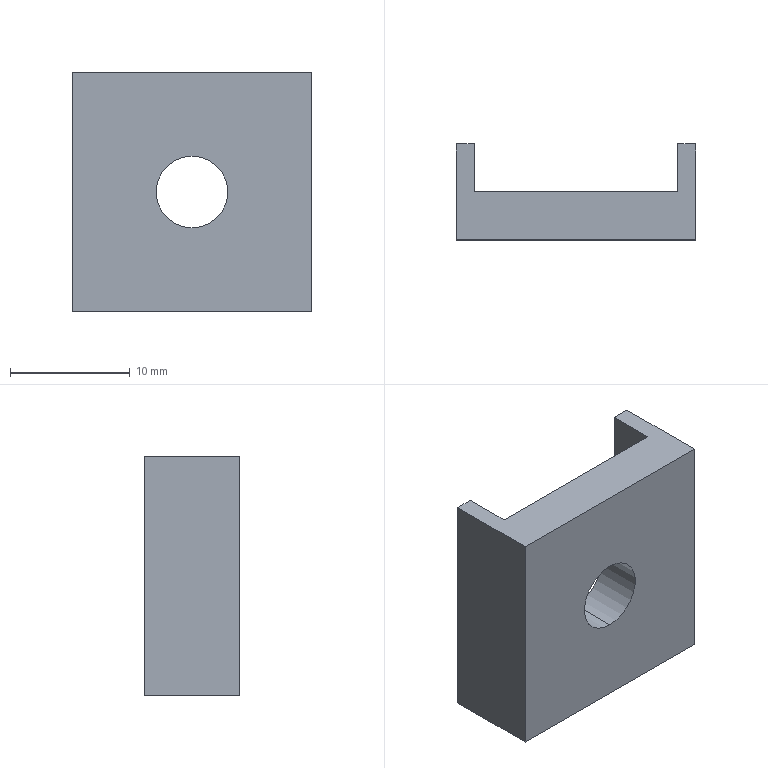Part | STEP file | 开关-2 | 1 solid | 12 faces | box 20 x 8 x 20 mm | volume 1727 mm3 | plane 10 | cylinder 2 | commonest cylinder face diameters 6 x2
STEP:
#1=CARTESIAN_POINT('',(0.,0.,0.));
#2=DIRECTION('',(0.,0.,1.));
#3=DIRECTION('',(1.,0.,0.));
#4=AXIS2_PLACEMENT_3D('',#1,#2,#3);
#5=CARTESIAN_POINT('',(0.,4.,-3.));
#6=VERTEX_POINT('',#5);
#7=CARTESIAN_POINT('',(0.,0.,-3.));
#8=VERTEX_POINT('',#7);
#9=CARTESIAN_POINT('',(0.,8.001,-3.));
#10=DIRECTION('',(0.,-1.,0.));
#11=VECTOR('',#10,1.);
#12=LINE('',#9,#11);
#13=CARTESIAN_POINT('',(0.,8.001,0.));
#14=DIRECTION('',(0.,-1.,0.));
#15=DIRECTION('',(0.,0.,-1.));
#16=AXIS2_PLACEMENT_3D('',#13,#14,#15);
#17=CYLINDRICAL_SURFACE('',#16,3.);
#18=CARTESIAN_POINT('',(6.283,0.));
#19=DIRECTION('',(0.,1.));
#20=VECTOR('',#19,1.);
#21=LINE('',#18,#20);
#22=(GEOMETRIC_REPRESENTATION_CONTEXT(2)PARAMETRIC_REPRESENTATION_CONTEXT()REPRESENTATION_CONTEXT('',''));
#23=DEFINITIONAL_REPRESENTATION('',(#21),#22);
#24=PCURVE('',#17,#23);
#25=CARTESIAN_POINT('',(0.,8.001,0.));
#26=DIRECTION('',(0.,-1.,0.));
#27=DIRECTION('',(0.,0.,-1.));
#28=AXIS2_PLACEMENT_3D('',#25,#26,#27);
#29=CYLINDRICAL_SURFACE('',#28,3.);
#30=CARTESIAN_POINT('',(0.,0.));
#31=DIRECTION('',(0.,1.));
#32=VECTOR('',#31,1.);
#33=LINE('',#30,#32);
#34=(GEOMETRIC_REPRESENTATION_CONTEXT(2)PARAMETRIC_REPRESENTATION_CONTEXT()REPRESENTATION_CONTEXT('',''));
#35=DEFINITIONAL_REPRESENTATION('',(#33),#34);
#36=PCURVE('',#29,#35);
#37=SURFACE_CURVE('',#12,(#24,#36),.PCURVE_S1.);
#38=EDGE_CURVE('',#6,#8,#37,.T.);
#39=ORIENTED_EDGE('',*,*,#38,.T.);
#40=CARTESIAN_POINT('',(0.,0.,3.));
#41=VERTEX_POINT('',#40);
#42=CARTESIAN_POINT('',(0.,0.,0.));
#43=DIRECTION('',(0.,-1.,0.));
#44=DIRECTION('',(0.,0.,-1.));
#45=AXIS2_PLACEMENT_3D('',#42,#43,#44);
#46=CIRCLE('',#45,3.);
#47=CARTESIAN_POINT('',(0.,8.001));
#48=DIRECTION('',(1.,0.));
#49=VECTOR('',#48,1.);
#50=LINE('',#47,#49);
#51=(GEOMETRIC_REPRESENTATION_CONTEXT(2)PARAMETRIC_REPRESENTATION_CONTEXT()REPRESENTATION_CONTEXT('',''));
#52=DEFINITIONAL_REPRESENTATION('',(#50),#51);
#53=PCURVE('',#17,#52);
#54=CARTESIAN_POINT('',(0.,0.,0.));
#55=DIRECTION('',(0.,-1.,0.));
#56=DIRECTION('',(0.,0.,-1.));
#57=AXIS2_PLACEMENT_3D('',#54,#55,#56);
#58=PLANE('',#57);
#59=CARTESIAN_POINT('',(0.,0.));
#60=DIRECTION('',(1.,0.));
#61=AXIS2_PLACEMENT_2D('',#59,#60);
#62=CIRCLE('',#61,3.);
#63=(GEOMETRIC_REPRESENTATION_CONTEXT(2)PARAMETRIC_REPRESENTATION_CONTEXT()REPRESENTATION_CONTEXT('',''));
#64=DEFINITIONAL_REPRESENTATION('',(#62),#63);
#65=PCURVE('',#58,#64);
#66=SURFACE_CURVE('',#46,(#53,#65),.PCURVE_S1.);
#67=EDGE_CURVE('',#41,#8,#66,.T.);
#68=ORIENTED_EDGE('',*,*,#67,.F.);
#69=CARTESIAN_POINT('',(0.,4.,3.));
#70=VERTEX_POINT('',#69);
#71=CARTESIAN_POINT('',(0.,8.001,3.));
#72=DIRECTION('',(0.,-1.,0.));
#73=VECTOR('',#72,1.);
#74=LINE('',#71,#73);
#75=CARTESIAN_POINT('',(3.142,0.));
#76=DIRECTION('',(0.,1.));
#77=VECTOR('',#76,1.);
#78=LINE('',#75,#77);
#79=(GEOMETRIC_REPRESENTATION_CONTEXT(2)PARAMETRIC_REPRESENTATION_CONTEXT()REPRESENTATION_CONTEXT('',''));
#80=DEFINITIONAL_REPRESENTATION('',(#78),#79);
#81=PCURVE('',#17,#80);
#82=CARTESIAN_POINT('',(3.142,0.));
#83=DIRECTION('',(0.,1.));
#84=VECTOR('',#83,1.);
#85=LINE('',#82,#84);
#86=(GEOMETRIC_REPRESENTATION_CONTEXT(2)PARAMETRIC_REPRESENTATION_CONTEXT()REPRESENTATION_CONTEXT('',''));
#87=DEFINITIONAL_REPRESENTATION('',(#85),#86);
#88=PCURVE('',#29,#87);
#89=SURFACE_CURVE('',#74,(#81,#88),.PCURVE_S1.);
#90=EDGE_CURVE('',#70,#41,#89,.T.);
#91=ORIENTED_EDGE('',*,*,#90,.F.);
#92=CARTESIAN_POINT('',(0.,4.,0.));
#93=DIRECTION('',(0.,1.,0.));
#94=DIRECTION('',(0.,0.,-1.));
#95=AXIS2_PLACEMENT_3D('',#92,#93,#94);
#96=CIRCLE('',#95,3.);
#97=CARTESIAN_POINT('',(6.283,4.001));
#98=DIRECTION('',(-1.,0.));
#99=VECTOR('',#98,1.);
#100=LINE('',#97,#99);
#101=(GEOMETRIC_REPRESENTATION_CONTEXT(2)PARAMETRIC_REPRESENTATION_CONTEXT()REPRESENTATION_CONTEXT('',''));
#102=DEFINITIONAL_REPRESENTATION('',(#100),#101);
#103=PCURVE('',#17,#102);
#104=CARTESIAN_POINT('',(-8.5,4.,-10.));
#105=DIRECTION('',(0.,-1.,0.));
#106=DIRECTION('',(0.,0.,-1.));
#107=AXIS2_PLACEMENT_3D('',#104,#105,#106);
#108=PLANE('',#107);
#109=CARTESIAN_POINT('',(-7.,8.5));
#110=CARTESIAN_POINT('',(-7.,3.304));
#111=CARTESIAN_POINT('',(-11.5,5.902));
#112=CARTESIAN_POINT('',(-16.,8.5));
#113=CARTESIAN_POINT('',(-11.5,11.098));
#114=CARTESIAN_POINT('',(-7.,13.696));
#115=CARTESIAN_POINT('',(-7.,8.5));
#116=(BOUNDED_CURVE()B_SPLINE_CURVE(2,(#109,#110,#111,#112,#113,#114,#115),.UNSPECIFIED.,.T.,.F.)B_SPLINE_CURVE_WITH_KNOTS((1,2,2,2,2,1),(-2.094,0.,2.094,4.189,6.283,8.378),.UNSPECIFIED.)CURVE()GEOMETRIC_REPRESENTATION_ITEM()RATIONAL_B_SPLINE_CURVE((1.,0.5,1.,0.5,1.,0.5,1.))REPRESENTATION_ITEM(''));
#117=(GEOMETRIC_REPRESENTATION_CONTEXT(2)PARAMETRIC_REPRESENTATION_CONTEXT()REPRESENTATION_CONTEXT('',''));
#118=DEFINITIONAL_REPRESENTATION('',(#116),#117);
#119=PCURVE('',#108,#118);
#120=SURFACE_CURVE('',#96,(#103,#119),.PCURVE_S1.);
#121=EDGE_CURVE('',#6,#70,#120,.T.);
#122=ORIENTED_EDGE('',*,*,#121,.F.);
#123=EDGE_LOOP('',(#39,#68,#91,#122));
#124=FACE_BOUND('',#123,.F.);
#125=ADVANCED_FACE('',(#124),#17,.F.);
#126=CARTESIAN_POINT('',(-10.,8.,10.));
#127=VERTEX_POINT('',#126);
#128=CARTESIAN_POINT('',(-8.5,8.,10.));
#129=VERTEX_POINT('',#128);
#130=CARTESIAN_POINT('',(-10.,8.,10.));
#131=DIRECTION('',(1.,0.,0.));
#132=VECTOR('',#131,1.);
#133=LINE('',#130,#132);
#134=CARTESIAN_POINT('',(0.,8.,0.));
#135=DIRECTION('',(0.,-1.,0.));
#136=DIRECTION('',(0.,0.,-1.));
#137=AXIS2_PLACEMENT_3D('',#134,#135,#136);
#138=PLANE('',#137);
#139=CARTESIAN_POINT('',(-10.,-10.));
#140=DIRECTION('',(0.,1.));
#141=VECTOR('',#140,1.);
#142=LINE('',#139,#141);
#143=(GEOMETRIC_REPRESENTATION_CONTEXT(2)PARAMETRIC_REPRESENTATION_CONTEXT()REPRESENTATION_CONTEXT('',''));
#144=DEFINITIONAL_REPRESENTATION('',(#142),#143);
#145=PCURVE('',#138,#144);
#146=CARTESIAN_POINT('',(-10.,8.,10.));
#147=DIRECTION('',(0.,0.,-1.));
#148=DIRECTION('',(-1.,0.,0.));
#149=AXIS2_PLACEMENT_3D('',#146,#147,#148);
#150=PLANE('',#149);
#151=CARTESIAN_POINT('',(0.,0.));
#152=DIRECTION('',(-1.,0.));
#153=VECTOR('',#152,1.);
#154=LINE('',#151,#153);
#155=(GEOMETRIC_REPRESENTATION_CONTEXT(2)PARAMETRIC_REPRESENTATION_CONTEXT()REPRESENTATION_CONTEXT('',''));
#156=DEFINITIONAL_REPRESENTATION('',(#154),#155);
#157=PCURVE('',#150,#156);
#158=SURFACE_CURVE('',#133,(#145,#157),.PCURVE_S1.);
#159=EDGE_CURVE('',#127,#129,#158,.T.);
#160=ORIENTED_EDGE('',*,*,#159,.T.);
#161=CARTESIAN_POINT('',(-8.5,8.,-10.));
#162=VERTEX_POINT('',#161);
#163=CARTESIAN_POINT('',(-8.5,8.,-10.));
#164=DIRECTION('',(0.,0.,1.));
#165=VECTOR('',#164,1.);
#166=LINE('',#163,#165);
#167=CARTESIAN_POINT('',(10.,-8.5));
#168=DIRECTION('',(-1.,0.));
#169=VECTOR('',#168,1.);
#170=LINE('',#167,#169);
#171=(GEOMETRIC_REPRESENTATION_CONTEXT(2)PARAMETRIC_REPRESENTATION_CONTEXT()REPRESENTATION_CONTEXT('',''));
#172=DEFINITIONAL_REPRESENTATION('',(#170),#171);
#173=PCURVE('',#138,#172);
#174=CARTESIAN_POINT('',(-8.5,8.,-10.));
#175=DIRECTION('',(-1.,0.,0.));
#176=DIRECTION('',(0.,0.,1.));
#177=AXIS2_PLACEMENT_3D('',#174,#175,#176);
#178=PLANE('',#177);
#179=CARTESIAN_POINT('',(0.,0.));
#180=DIRECTION('',(1.,0.));
#181=VECTOR('',#180,1.);
#182=LINE('',#179,#181);
#183=(GEOMETRIC_REPRESENTATION_CONTEXT(2)PARAMETRIC_REPRESENTATION_CONTEXT()REPRESENTATION_CONTEXT('',''));
#184=DEFINITIONAL_REPRESENTATION('',(#182),#183);
#185=PCURVE('',#178,#184);
#186=SURFACE_CURVE('',#166,(#173,#185),.PCURVE_S1.);
#187=EDGE_CURVE('',#162,#129,#186,.T.);
#188=ORIENTED_EDGE('',*,*,#187,.F.);
#189=CARTESIAN_POINT('',(-10.,8.,-10.));
#190=VERTEX_POINT('',#189);
#191=CARTESIAN_POINT('',(-10.,8.,-10.));
#192=DIRECTION('',(-1.,0.,0.));
#193=VECTOR('',#192,1.);
#194=LINE('',#191,#193);
#195=CARTESIAN_POINT('',(10.,-10.));
#196=DIRECTION('',(0.,-1.));
#197=VECTOR('',#196,1.);
#198=LINE('',#195,#197);
#199=(GEOMETRIC_REPRESENTATION_CONTEXT(2)PARAMETRIC_REPRESENTATION_CONTEXT()REPRESENTATION_CONTEXT('',''));
#200=DEFINITIONAL_REPRESENTATION('',(#198),#199);
#201=PCURVE('',#138,#200);
#202=CARTESIAN_POINT('',(-10.,8.,-10.));
#203=DIRECTION('',(0.,0.,1.));
#204=DIRECTION('',(1.,0.,0.));
#205=AXIS2_PLACEMENT_3D('',#202,#203,#204);
#206=PLANE('',#205);
#207=CARTESIAN_POINT('',(0.,0.));
#208=DIRECTION('',(-1.,0.));
#209=VECTOR('',#208,1.);
#210=LINE('',#207,#209);
#211=(GEOMETRIC_REPRESENTATION_CONTEXT(2)PARAMETRIC_REPRESENTATION_CONTEXT()REPRESENTATION_CONTEXT('',''));
#212=DEFINITIONAL_REPRESENTATION('',(#210),#211);
#213=PCURVE('',#206,#212);
#214=SURFACE_CURVE('',#194,(#201,#213),.PCURVE_S1.);
#215=EDGE_CURVE('',#162,#190,#214,.T.);
#216=ORIENTED_EDGE('',*,*,#215,.T.);
#217=CARTESIAN_POINT('',(-10.,8.,10.));
#218=DIRECTION('',(0.,0.,1.));
#219=VECTOR('',#218,1.);
#220=LINE('',#217,#219);
#221=CARTESIAN_POINT('',(-10.,-10.));
#222=DIRECTION('',(-1.,0.));
#223=VECTOR('',#222,1.);
#224=LINE('',#221,#223);
#225=(GEOMETRIC_REPRESENTATION_CONTEXT(2)PARAMETRIC_REPRESENTATION_CONTEXT()REPRESENTATION_CONTEXT('',''));
#226=DEFINITIONAL_REPRESENTATION('',(#224),#225);
#227=PCURVE('',#138,#226);
#228=CARTESIAN_POINT('',(-10.,8.,10.));
#229=DIRECTION('',(1.,0.,0.));
#230=DIRECTION('',(0.,0.,-1.));
#231=AXIS2_PLACEMENT_3D('',#228,#229,#230);
#232=PLANE('',#231);
#233=CARTESIAN_POINT('',(0.,0.));
#234=DIRECTION('',(-1.,0.));
#235=VECTOR('',#234,1.);
#236=LINE('',#233,#235);
#237=(GEOMETRIC_REPRESENTATION_CONTEXT(2)PARAMETRIC_REPRESENTATION_CONTEXT()REPRESENTATION_CONTEXT('',''));
#238=DEFINITIONAL_REPRESENTATION('',(#236),#237);
#239=PCURVE('',#232,#238);
#240=SURFACE_CURVE('',#220,(#227,#239),.PCURVE_S1.);
#241=EDGE_CURVE('',#190,#127,#240,.T.);
#242=ORIENTED_EDGE('',*,*,#241,.T.);
#243=EDGE_LOOP('',(#160,#188,#216,#242));
#244=FACE_BOUND('',#243,.T.);
#245=ADVANCED_FACE('',(#244),#138,.F.);
#246=CARTESIAN_POINT('',(10.,0.,10.));
#247=VERTEX_POINT('',#246);
#248=CARTESIAN_POINT('',(10.,0.,-10.));
#249=VERTEX_POINT('',#248);
#250=CARTESIAN_POINT('',(10.,0.,10.));
#251=DIRECTION('',(0.,0.,-1.));
#252=VECTOR('',#251,1.);
#253=LINE('',#250,#252);
#254=CARTESIAN_POINT('',(10.,8.,10.));
#255=DIRECTION('',(-1.,0.,0.));
#256=DIRECTION('',(0.,0.,1.));
#257=AXIS2_PLACEMENT_3D('',#254,#255,#256);
#258=PLANE('',#257);
#259=CARTESIAN_POINT('',(0.,-8.));
#260=DIRECTION('',(-1.,0.));
#261=VECTOR('',#260,1.);
#262=LINE('',#259,#261);
#263=(GEOMETRIC_REPRESENTATION_CONTEXT(2)PARAMETRIC_REPRESENTATION_CONTEXT()REPRESENTATION_CONTEXT('',''));
#264=DEFINITIONAL_REPRESENTATION('',(#262),#263);
#265=PCURVE('',#258,#264);
#266=CARTESIAN_POINT('',(-10.,10.));
#267=DIRECTION('',(1.,0.));
#268=VECTOR('',#267,1.);
#269=LINE('',#266,#268);
#270=(GEOMETRIC_REPRESENTATION_CONTEXT(2)PARAMETRIC_REPRESENTATION_CONTEXT()REPRESENTATION_CONTEXT('',''));
#271=DEFINITIONAL_REPRESENTATION('',(#269),#270);
#272=PCURVE('',#58,#271);
#273=SURFACE_CURVE('',#253,(#265,#272),.PCURVE_S1.);
#274=EDGE_CURVE('',#247,#249,#273,.T.);
#275=ORIENTED_EDGE('',*,*,#274,.T.);
#276=CARTESIAN_POINT('',(10.,8.,-10.));
#277=VERTEX_POINT('',#276);
#278=CARTESIAN_POINT('',(10.,8.,-10.));
#279=DIRECTION('',(0.,-1.,0.));
#280=VECTOR('',#279,1.);
#281=LINE('',#278,#280);
#282=CARTESIAN_POINT('',(-20.,0.));
#283=DIRECTION('',(0.,-1.));
#284=VECTOR('',#283,1.);
#285=LINE('',#282,#284);
#286=(GEOMETRIC_REPRESENTATION_CONTEXT(2)PARAMETRIC_REPRESENTATION_CONTEXT()REPRESENTATION_CONTEXT('',''));
#287=DEFINITIONAL_REPRESENTATION('',(#285),#286);
#288=PCURVE('',#258,#287);
#289=CARTESIAN_POINT('',(20.,0.));
#290=DIRECTION('',(0.,-1.));
#291=VECTOR('',#290,1.);
#292=LINE('',#289,#291);
#293=(GEOMETRIC_REPRESENTATION_CONTEXT(2)PARAMETRIC_REPRESENTATION_CONTEXT()REPRESENTATION_CONTEXT('',''));
#294=DEFINITIONAL_REPRESENTATION('',(#292),#293);
#295=PCURVE('',#206,#294);
#296=SURFACE_CURVE('',#281,(#288,#295),.PCURVE_S1.);
#297=EDGE_CURVE('',#277,#249,#296,.T.);
#298=ORIENTED_EDGE('',*,*,#297,.F.);
#299=CARTESIAN_POINT('',(10.,8.,10.));
#300=VERTEX_POINT('',#299);
#301=CARTESIAN_POINT('',(10.,8.,10.));
#302=DIRECTION('',(0.,0.,-1.));
#303=VECTOR('',#302,1.);
#304=LINE('',#301,#303);
#305=CARTESIAN_POINT('',(0.,0.));
#306=DIRECTION('',(-1.,0.));
#307=VECTOR('',#306,1.);
#308=LINE('',#305,#307);
#309=(GEOMETRIC_REPRESENTATION_CONTEXT(2)PARAMETRIC_REPRESENTATION_CONTEXT()REPRESENTATION_CONTEXT('',''));
#310=DEFINITIONAL_REPRESENTATION('',(#308),#309);
#311=PCURVE('',#258,#310);
#312=CARTESIAN_POINT('',(0.,8.,0.));
#313=DIRECTION('',(0.,-1.,0.));
#314=DIRECTION('',(0.,0.,-1.));
#315=AXIS2_PLACEMENT_3D('',#312,#313,#314);
#316=PLANE('',#315);
#317=CARTESIAN_POINT('',(-10.,10.));
#318=DIRECTION('',(1.,0.));
#319=VECTOR('',#318,1.);
#320=LINE('',#317,#319);
#321=(GEOMETRIC_REPRESENTATION_CONTEXT(2)PARAMETRIC_REPRESENTATION_CONTEXT()REPRESENTATION_CONTEXT('',''));
#322=DEFINITIONAL_REPRESENTATION('',(#320),#321);
#323=PCURVE('',#316,#322);
#324=SURFACE_CURVE('',#304,(#311,#323),.PCURVE_S1.);
#325=EDGE_CURVE('',#300,#277,#324,.T.);
#326=ORIENTED_EDGE('',*,*,#325,.F.);
#327=CARTESIAN_POINT('',(10.,8.,10.));
#328=DIRECTION('',(0.,-1.,0.));
#329=VECTOR('',#328,1.);
#330=LINE('',#327,#329);
#331=CARTESIAN_POINT('',(0.,0.));
#332=DIRECTION('',(0.,-1.));
#333=VECTOR('',#332,1.);
#334=LINE('',#331,#333);
#335=(GEOMETRIC_REPRESENTATION_CONTEXT(2)PARAMETRIC_REPRESENTATION_CONTEXT()REPRESENTATION_CONTEXT('',''));
#336=DEFINITIONAL_REPRESENTATION('',(#334),#335);
#337=PCURVE('',#258,#336);
#338=CARTESIAN_POINT('',(-20.,0.));
#339=DIRECTION('',(0.,-1.));
#340=VECTOR('',#339,1.);
#341=LINE('',#338,#340);
#342=(GEOMETRIC_REPRESENTATION_CONTEXT(2)PARAMETRIC_REPRESENTATION_CONTEXT()REPRESENTATION_CONTEXT('',''));
#343=DEFINITIONAL_REPRESENTATION('',(#341),#342);
#344=PCURVE('',#150,#343);
#345=SURFACE_CURVE('',#330,(#337,#344),.PCURVE_S1.);
#346=EDGE_CURVE('',#300,#247,#345,.T.);
#347=ORIENTED_EDGE('',*,*,#346,.T.);
#348=EDGE_LOOP('',(#275,#298,#326,#347));
#349=FACE_BOUND('',#348,.T.);
#350=ADVANCED_FACE('',(#349),#258,.F.);
#351=ORIENTED_EDGE('',*,*,#215,.F.);
#352=CARTESIAN_POINT('',(-8.5,4.,-10.));
#353=VERTEX_POINT('',#352);
#354=CARTESIAN_POINT('',(-8.5,8.,-10.));
#355=DIRECTION('',(0.,-1.,0.));
#356=VECTOR('',#355,1.);
#357=LINE('',#354,#356);
#358=CARTESIAN_POINT('',(1.5,0.));
#359=DIRECTION('',(0.,-1.));
#360=VECTOR('',#359,1.);
#361=LINE('',#358,#360);
#362=(GEOMETRIC_REPRESENTATION_CONTEXT(2)PARAMETRIC_REPRESENTATION_CONTEXT()REPRESENTATION_CONTEXT('',''));
#363=DEFINITIONAL_REPRESENTATION('',(#361),#362);
#364=PCURVE('',#206,#363);
#365=CARTESIAN_POINT('',(0.,0.));
#366=DIRECTION('',(0.,-1.));
#367=VECTOR('',#366,1.);
#368=LINE('',#365,#367);
#369=(GEOMETRIC_REPRESENTATION_CONTEXT(2)PARAMETRIC_REPRESENTATION_CONTEXT()REPRESENTATION_CONTEXT('',''));
#370=DEFINITIONAL_REPRESENTATION('',(#368),#369);
#371=PCURVE('',#178,#370);
#372=SURFACE_CURVE('',#357,(#364,#371),.PCURVE_S1.);
#373=EDGE_CURVE('',#162,#353,#372,.T.);
#374=ORIENTED_EDGE('',*,*,#373,.T.);
#375=CARTESIAN_POINT('',(8.5,4.,-10.));
#376=VERTEX_POINT('',#375);
#377=CARTESIAN_POINT('',(-8.5,4.,-10.));
#378=DIRECTION('',(1.,0.,0.));
#379=VECTOR('',#378,1.);
#380=LINE('',#377,#379);
#381=CARTESIAN_POINT('',(1.5,-4.));
#382=DIRECTION('',(1.,0.));
#383=VECTOR('',#382,1.);
#384=LINE('',#381,#383);
#385=(GEOMETRIC_REPRESENTATION_CONTEXT(2)PARAMETRIC_REPRESENTATION_CONTEXT()REPRESENTATION_CONTEXT('',''));
#386=DEFINITIONAL_REPRESENTATION('',(#384),#385);
#387=PCURVE('',#206,#386);
#388=CARTESIAN_POINT('',(0.,0.));
#389=DIRECTION('',(0.,1.));
#390=VECTOR('',#389,1.);
#391=LINE('',#388,#390);
#392=(GEOMETRIC_REPRESENTATION_CONTEXT(2)PARAMETRIC_REPRESENTATION_CONTEXT()REPRESENTATION_CONTEXT('',''));
#393=DEFINITIONAL_REPRESENTATION('',(#391),#392);
#394=PCURVE('',#108,#393);
#395=SURFACE_CURVE('',#380,(#387,#394),.PCURVE_S1.);
#396=EDGE_CURVE('',#353,#376,#395,.T.);
#397=ORIENTED_EDGE('',*,*,#396,.T.);
#398=CARTESIAN_POINT('',(8.5,8.,-10.));
#399=VERTEX_POINT('',#398);
#400=CARTESIAN_POINT('',(8.5,8.,-10.));
#401=DIRECTION('',(0.,1.,0.));
#402=VECTOR('',#401,1.);
#403=LINE('',#400,#402);
#404=CARTESIAN_POINT('',(18.5,0.));
#405=DIRECTION('',(0.,1.));
#406=VECTOR('',#405,1.);
#407=LINE('',#404,#406);
#408=(GEOMETRIC_REPRESENTATION_CONTEXT(2)PARAMETRIC_REPRESENTATION_CONTEXT()REPRESENTATION_CONTEXT('',''));
#409=DEFINITIONAL_REPRESENTATION('',(#407),#408);
#410=PCURVE('',#206,#409);
#411=CARTESIAN_POINT('',(8.5,8.,-10.));
#412=DIRECTION('',(1.,0.,0.));
#413=DIRECTION('',(0.,0.,-1.));
#414=AXIS2_PLACEMENT_3D('',#411,#412,#413);
#415=PLANE('',#414);
#416=CARTESIAN_POINT('',(0.,0.));
#417=DIRECTION('',(0.,1.));
#418=VECTOR('',#417,1.);
#419=LINE('',#416,#418);
#420=(GEOMETRIC_REPRESENTATION_CONTEXT(2)PARAMETRIC_REPRESENTATION_CONTEXT()REPRESENTATION_CONTEXT('',''));
#421=DEFINITIONAL_REPRESENTATION('',(#419),#420);
#422=PCURVE('',#415,#421);
#423=SURFACE_CURVE('',#403,(#410,#422),.PCURVE_S1.);
#424=EDGE_CURVE('',#376,#399,#423,.T.);
#425=ORIENTED_EDGE('',*,*,#424,.T.);
#426=CARTESIAN_POINT('',(-10.,8.,-10.));
#427=DIRECTION('',(-1.,0.,0.));
#428=VECTOR('',#427,1.);
#429=LINE('',#426,#428);
#430=CARTESIAN_POINT('',(0.,0.));
#431=DIRECTION('',(-1.,0.));
#432=VECTOR('',#431,1.);
#433=LINE('',#430,#432);
#434=(GEOMETRIC_REPRESENTATION_CONTEXT(2)PARAMETRIC_REPRESENTATION_CONTEXT()REPRESENTATION_CONTEXT('',''));
#435=DEFINITIONAL_REPRESENTATION('',(#433),#434);
#436=PCURVE('',#206,#435);
#437=CARTESIAN_POINT('',(10.,-10.));
#438=DIRECTION('',(0.,-1.));
#439=VECTOR('',#438,1.);
#440=LINE('',#437,#439);
#441=(GEOMETRIC_REPRESENTATION_CONTEXT(2)PARAMETRIC_REPRESENTATION_CONTEXT()REPRESENTATION_CONTEXT('',''));
#442=DEFINITIONAL_REPRESENTATION('',(#440),#441);
#443=PCURVE('',#316,#442);
#444=SURFACE_CURVE('',#429,(#436,#443),.PCURVE_S1.);
#445=EDGE_CURVE('',#277,#399,#444,.T.);
#446=ORIENTED_EDGE('',*,*,#445,.F.);
#447=ORIENTED_EDGE('',*,*,#297,.T.);
#448=CARTESIAN_POINT('',(-10.,0.,-10.));
#449=VERTEX_POINT('',#448);
#450=CARTESIAN_POINT('',(-10.,0.,-10.));
#451=DIRECTION('',(-1.,0.,0.));
#452=VECTOR('',#451,1.);
#453=LINE('',#450,#452);
#454=CARTESIAN_POINT('',(0.,-8.));
#455=DIRECTION('',(-1.,0.));
#456=VECTOR('',#455,1.);
#457=LINE('',#454,#456);
#458=(GEOMETRIC_REPRESENTATION_CONTEXT(2)PARAMETRIC_REPRESENTATION_CONTEXT()REPRESENTATION_CONTEXT('',''));
#459=DEFINITIONAL_REPRESENTATION('',(#457),#458);
#460=PCURVE('',#206,#459);
#461=CARTESIAN_POINT('',(10.,-10.));
#462=DIRECTION('',(0.,-1.));
#463=VECTOR('',#462,1.);
#464=LINE('',#461,#463);
#465=(GEOMETRIC_REPRESENTATION_CONTEXT(2)PARAMETRIC_REPRESENTATION_CONTEXT()REPRESENTATION_CONTEXT('',''));
#466=DEFINITIONAL_REPRESENTATION('',(#464),#465);
#467=PCURVE('',#58,#466);
#468=SURFACE_CURVE('',#453,(#460,#467),.PCURVE_S1.);
#469=EDGE_CURVE('',#249,#449,#468,.T.);
#470=ORIENTED_EDGE('',*,*,#469,.T.);
#471=CARTESIAN_POINT('',(-10.,8.,-10.));
#472=DIRECTION('',(0.,-1.,0.));
#473=VECTOR('',#472,1.);
#474=LINE('',#471,#473);
#475=CARTESIAN_POINT('',(0.,0.));
#476=DIRECTION('',(0.,-1.));
#477=VECTOR('',#476,1.);
#478=LINE('',#475,#477);
#479=(GEOMETRIC_REPRESENTATION_CONTEXT(2)PARAMETRIC_REPRESENTATION_CONTEXT()REPRESENTATION_CONTEXT('',''));
#480=DEFINITIONAL_REPRESENTATION('',(#478),#479);
#481=PCURVE('',#206,#480);
#482=CARTESIAN_POINT('',(20.,0.));
#483=DIRECTION('',(0.,-1.));
#484=VECTOR('',#483,1.);
#485=LINE('',#482,#484);
#486=(GEOMETRIC_REPRESENTATION_CONTEXT(2)PARAMETRIC_REPRESENTATION_CONTEXT()REPRESENTATION_CONTEXT('',''));
#487=DEFINITIONAL_REPRESENTATION('',(#485),#486);
#488=PCURVE('',#232,#487);
#489=SURFACE_CURVE('',#474,(#481,#488),.PCURVE_S1.);
#490=EDGE_CURVE('',#190,#449,#489,.T.);
#491=ORIENTED_EDGE('',*,*,#490,.F.);
#492=EDGE_LOOP('',(#351,#374,#397,#425,#446,#447,#470,#491));
#493=FACE_BOUND('',#492,.T.);
#494=ADVANCED_FACE('',(#493),#206,.F.);
#495=CARTESIAN_POINT('',(-10.,0.,10.));
#496=VERTEX_POINT('',#495);
#497=CARTESIAN_POINT('',(-10.,0.,10.));
#498=DIRECTION('',(0.,0.,1.));
#499=VECTOR('',#498,1.);
#500=LINE('',#497,#499);
#501=CARTESIAN_POINT('',(0.,-8.));
#502=DIRECTION('',(-1.,0.));
#503=VECTOR('',#502,1.);
#504=LINE('',#501,#503);
#505=(GEOMETRIC_REPRESENTATION_CONTEXT(2)PARAMETRIC_REPRESENTATION_CONTEXT()REPRESENTATION_CONTEXT('',''));
#506=DEFINITIONAL_REPRESENTATION('',(#504),#505);
#507=PCURVE('',#232,#506);
#508=CARTESIAN_POINT('',(-10.,-10.));
#509=DIRECTION('',(-1.,0.));
#510=VECTOR('',#509,1.);
#511=LINE('',#508,#510);
#512=(GEOMETRIC_REPRESENTATION_CONTEXT(2)PARAMETRIC_REPRESENTATION_CONTEXT()REPRESENTATION_CONTEXT('',''));
#513=DEFINITIONAL_REPRESENTATION('',(#511),#512);
#514=PCURVE('',#58,#513);
#515=SURFACE_CURVE('',#500,(#507,#514),.PCURVE_S1.);
#516=EDGE_CURVE('',#449,#496,#515,.T.);
#517=ORIENTED_EDGE('',*,*,#516,.T.);
#518=CARTESIAN_POINT('',(-10.,8.,10.));
#519=DIRECTION('',(0.,-1.,0.));
#520=VECTOR('',#519,1.);
#521=LINE('',#518,#520);
#522=CARTESIAN_POINT('',(0.,0.));
#523=DIRECTION('',(0.,-1.));
#524=VECTOR('',#523,1.);
#525=LINE('',#522,#524);
#526=(GEOMETRIC_REPRESENTATION_CONTEXT(2)PARAMETRIC_REPRESENTATION_CONTEXT()REPRESENTATION_CONTEXT('',''));
#527=DEFINITIONAL_REPRESENTATION('',(#525),#526);
#528=PCURVE('',#232,#527);
#529=CARTESIAN_POINT('',(0.,0.));
#530=DIRECTION('',(0.,-1.));
#531=VECTOR('',#530,1.);
#532=LINE('',#529,#531);
#533=(GEOMETRIC_REPRESENTATION_CONTEXT(2)PARAMETRIC_REPRESENTATION_CONTEXT()REPRESENTATION_CONTEXT('',''));
#534=DEFINITIONAL_REPRESENTATION('',(#532),#533);
#535=PCURVE('',#150,#534);
#536=SURFACE_CURVE('',#521,(#528,#535),.PCURVE_S1.);
#537=EDGE_CURVE('',#127,#496,#536,.T.);
#538=ORIENTED_EDGE('',*,*,#537,.F.);
#539=ORIENTED_EDGE('',*,*,#241,.F.);
#540=ORIENTED_EDGE('',*,*,#490,.T.);
#541=EDGE_LOOP('',(#517,#538,#539,#540));
#542=FACE_BOUND('',#541,.T.);
#543=ADVANCED_FACE('',(#542),#232,.F.);
#544=CARTESIAN_POINT('',(-8.5,4.,10.));
#545=VERTEX_POINT('',#544);
#546=CARTESIAN_POINT('',(8.5,4.,10.));
#547=VERTEX_POINT('',#546);
#548=CARTESIAN_POINT('',(-8.5,4.,10.));
#549=DIRECTION('',(1.,0.,0.));
#550=VECTOR('',#549,1.);
#551=LINE('',#548,#550);
#552=CARTESIAN_POINT('',(-1.5,-4.));
#553=DIRECTION('',(-1.,0.));
#554=VECTOR('',#553,1.);
#555=LINE('',#552,#554);
#556=(GEOMETRIC_REPRESENTATION_CONTEXT(2)PARAMETRIC_REPRESENTATION_CONTEXT()REPRESENTATION_CONTEXT('',''));
#557=DEFINITIONAL_REPRESENTATION('',(#555),#556);
#558=PCURVE('',#150,#557);
#559=CARTESIAN_POINT('',(-20.,0.));
#560=DIRECTION('',(0.,1.));
#561=VECTOR('',#560,1.);
#562=LINE('',#559,#561);
#563=(GEOMETRIC_REPRESENTATION_CONTEXT(2)PARAMETRIC_REPRESENTATION_CONTEXT()REPRESENTATION_CONTEXT('',''));
#564=DEFINITIONAL_REPRESENTATION('',(#562),#563);
#565=PCURVE('',#108,#564);
#566=SURFACE_CURVE('',#551,(#558,#565),.PCURVE_S1.);
#567=EDGE_CURVE('',#545,#547,#566,.T.);
#568=ORIENTED_EDGE('',*,*,#567,.F.);
#569=CARTESIAN_POINT('',(-8.5,8.,10.));
#570=DIRECTION('',(0.,-1.,0.));
#571=VECTOR('',#570,1.);
#572=LINE('',#569,#571);
#573=CARTESIAN_POINT('',(-1.5,0.));
#574=DIRECTION('',(0.,-1.));
#575=VECTOR('',#574,1.);
#576=LINE('',#573,#575);
#577=(GEOMETRIC_REPRESENTATION_CONTEXT(2)PARAMETRIC_REPRESENTATION_CONTEXT()REPRESENTATION_CONTEXT('',''));
#578=DEFINITIONAL_REPRESENTATION('',(#576),#577);
#579=PCURVE('',#150,#578);
#580=CARTESIAN_POINT('',(20.,0.));
#581=DIRECTION('',(0.,-1.));
#582=VECTOR('',#581,1.);
#583=LINE('',#580,#582);
#584=(GEOMETRIC_REPRESENTATION_CONTEXT(2)PARAMETRIC_REPRESENTATION_CONTEXT()REPRESENTATION_CONTEXT('',''));
#585=DEFINITIONAL_REPRESENTATION('',(#583),#584);
#586=PCURVE('',#178,#585);
#587=SURFACE_CURVE('',#572,(#579,#586),.PCURVE_S1.);
#588=EDGE_CURVE('',#129,#545,#587,.T.);
#589=ORIENTED_EDGE('',*,*,#588,.F.);
#590=ORIENTED_EDGE('',*,*,#159,.F.);
#591=ORIENTED_EDGE('',*,*,#537,.T.);
#592=CARTESIAN_POINT('',(-10.,0.,10.));
#593=DIRECTION('',(1.,0.,0.));
#594=VECTOR('',#593,1.);
#595=LINE('',#592,#594);
#596=CARTESIAN_POINT('',(0.,-8.));
#597=DIRECTION('',(-1.,0.));
#598=VECTOR('',#597,1.);
#599=LINE('',#596,#598);
#600=(GEOMETRIC_REPRESENTATION_CONTEXT(2)PARAMETRIC_REPRESENTATION_CONTEXT()REPRESENTATION_CONTEXT('',''));
#601=DEFINITIONAL_REPRESENTATION('',(#599),#600);
#602=PCURVE('',#150,#601);
#603=CARTESIAN_POINT('',(-10.,-10.));
#604=DIRECTION('',(0.,1.));
#605=VECTOR('',#604,1.);
#606=LINE('',#603,#605);
#607=(GEOMETRIC_REPRESENTATION_CONTEXT(2)PARAMETRIC_REPRESENTATION_CONTEXT()REPRESENTATION_CONTEXT('',''));
#608=DEFINITIONAL_REPRESENTATION('',(#606),#607);
#609=PCURVE('',#58,#608);
#610=SURFACE_CURVE('',#595,(#602,#609),.PCURVE_S1.);
#611=EDGE_CURVE('',#496,#247,#610,.T.);
#612=ORIENTED_EDGE('',*,*,#611,.T.);
#613=ORIENTED_EDGE('',*,*,#346,.F.);
#614=CARTESIAN_POINT('',(8.5,8.,10.));
#615=VERTEX_POINT('',#614);
#616=CARTESIAN_POINT('',(-10.,8.,10.));
#617=DIRECTION('',(1.,0.,0.));
#618=VECTOR('',#617,1.);
#619=LINE('',#616,#618);
#620=CARTESIAN_POINT('',(0.,0.));
#621=DIRECTION('',(-1.,0.));
#622=VECTOR('',#621,1.);
#623=LINE('',#620,#622);
#624=(GEOMETRIC_REPRESENTATION_CONTEXT(2)PARAMETRIC_REPRESENTATION_CONTEXT()REPRESENTATION_CONTEXT('',''));
#625=DEFINITIONAL_REPRESENTATION('',(#623),#624);
#626=PCURVE('',#150,#625);
#627=CARTESIAN_POINT('',(-10.,-10.));
#628=DIRECTION('',(0.,1.));
#629=VECTOR('',#628,1.);
#630=LINE('',#627,#629);
#631=(GEOMETRIC_REPRESENTATION_CONTEXT(2)PARAMETRIC_REPRESENTATION_CONTEXT()REPRESENTATION_CONTEXT('',''));
#632=DEFINITIONAL_REPRESENTATION('',(#630),#631);
#633=PCURVE('',#316,#632);
#634=SURFACE_CURVE('',#619,(#626,#633),.PCURVE_S1.);
#635=EDGE_CURVE('',#615,#300,#634,.T.);
#636=ORIENTED_EDGE('',*,*,#635,.F.);
#637=CARTESIAN_POINT('',(8.5,8.,10.));
#638=DIRECTION('',(0.,1.,0.));
#639=VECTOR('',#638,1.);
#640=LINE('',#637,#639);
#641=CARTESIAN_POINT('',(-18.5,0.));
#642=DIRECTION('',(0.,1.));
#643=VECTOR('',#642,1.);
#644=LINE('',#641,#643);
#645=(GEOMETRIC_REPRESENTATION_CONTEXT(2)PARAMETRIC_REPRESENTATION_CONTEXT()REPRESENTATION_CONTEXT('',''));
#646=DEFINITIONAL_REPRESENTATION('',(#644),#645);
#647=PCURVE('',#150,#646);
#648=CARTESIAN_POINT('',(-20.,0.));
#649=DIRECTION('',(0.,1.));
#650=VECTOR('',#649,1.);
#651=LINE('',#648,#650);
#652=(GEOMETRIC_REPRESENTATION_CONTEXT(2)PARAMETRIC_REPRESENTATION_CONTEXT()REPRESENTATION_CONTEXT('',''));
#653=DEFINITIONAL_REPRESENTATION('',(#651),#652);
#654=PCURVE('',#415,#653);
#655=SURFACE_CURVE('',#640,(#647,#654),.PCURVE_S1.);
#656=EDGE_CURVE('',#547,#615,#655,.T.);
#657=ORIENTED_EDGE('',*,*,#656,.F.);
#658=EDGE_LOOP('',(#568,#589,#590,#591,#612,#613,#636,#657));
#659=FACE_BOUND('',#658,.T.);
#660=ADVANCED_FACE('',(#659),#150,.F.);
#661=ORIENTED_EDGE('',*,*,#445,.T.);
#662=CARTESIAN_POINT('',(8.5,8.,-10.));
#663=DIRECTION('',(0.,0.,1.));
#664=VECTOR('',#663,1.);
#665=LINE('',#662,#664);
#666=CARTESIAN_POINT('',(10.,8.5));
#667=DIRECTION('',(-1.,0.));
#668=VECTOR('',#667,1.);
#669=LINE('',#666,#668);
#670=(GEOMETRIC_REPRESENTATION_CONTEXT(2)PARAMETRIC_REPRESENTATION_CONTEXT()REPRESENTATION_CONTEXT('',''));
#671=DEFINITIONAL_REPRESENTATION('',(#669),#670);
#672=PCURVE('',#316,#671);
#673=CARTESIAN_POINT('',(0.,0.));
#674=DIRECTION('',(-1.,0.));
#675=VECTOR('',#674,1.);
#676=LINE('',#673,#675);
#677=(GEOMETRIC_REPRESENTATION_CONTEXT(2)PARAMETRIC_REPRESENTATION_CONTEXT()REPRESENTATION_CONTEXT('',''));
#678=DEFINITIONAL_REPRESENTATION('',(#676),#677);
#679=PCURVE('',#415,#678);
#680=SURFACE_CURVE('',#665,(#672,#679),.PCURVE_S1.);
#681=EDGE_CURVE('',#399,#615,#680,.T.);
#682=ORIENTED_EDGE('',*,*,#681,.T.);
#683=ORIENTED_EDGE('',*,*,#635,.T.);
#684=ORIENTED_EDGE('',*,*,#325,.T.);
#685=EDGE_LOOP('',(#661,#682,#683,#684));
#686=FACE_BOUND('',#685,.T.);
#687=ADVANCED_FACE('',(#686),#316,.F.);
#688=CARTESIAN_POINT('',(0.,0.,0.));
#689=DIRECTION('',(0.,-1.,0.));
#690=DIRECTION('',(0.,0.,-1.));
#691=AXIS2_PLACEMENT_3D('',#688,#689,#690);
#692=CIRCLE('',#691,3.);
#693=CARTESIAN_POINT('',(0.,0.));
#694=DIRECTION('',(1.,0.));
#695=AXIS2_PLACEMENT_2D('',#693,#694);
#696=CIRCLE('',#695,3.);
#697=(GEOMETRIC_REPRESENTATION_CONTEXT(2)PARAMETRIC_REPRESENTATION_CONTEXT()REPRESENTATION_CONTEXT('',''));
#698=DEFINITIONAL_REPRESENTATION('',(#696),#697);
#699=PCURVE('',#58,#698);
#700=CARTESIAN_POINT('',(0.,8.001));
#701=DIRECTION('',(1.,0.));
#702=VECTOR('',#701,1.);
#703=LINE('',#700,#702);
#704=(GEOMETRIC_REPRESENTATION_CONTEXT(2)PARAMETRIC_REPRESENTATION_CONTEXT()REPRESENTATION_CONTEXT('',''));
#705=DEFINITIONAL_REPRESENTATION('',(#703),#704);
#706=PCURVE('',#29,#705);
#707=SURFACE_CURVE('',#692,(#699,#706),.PCURVE_S1.);
#708=EDGE_CURVE('',#8,#41,#707,.T.);
#709=ORIENTED_EDGE('',*,*,#708,.F.);
#710=ORIENTED_EDGE('',*,*,#67,.F.);
#711=EDGE_LOOP('',(#709,#710));
#712=FACE_BOUND('',#711,.T.);
#713=ORIENTED_EDGE('',*,*,#274,.F.);
#714=ORIENTED_EDGE('',*,*,#611,.F.);
#715=ORIENTED_EDGE('',*,*,#516,.F.);
#716=ORIENTED_EDGE('',*,*,#469,.F.);
#717=EDGE_LOOP('',(#713,#714,#715,#716));
#718=FACE_BOUND('',#717,.T.);
#719=ADVANCED_FACE('',(#712,#718),#58,.T.);
#720=ORIENTED_EDGE('',*,*,#588,.T.);
#721=CARTESIAN_POINT('',(-8.5,4.,-10.));
#722=DIRECTION('',(0.,0.,1.));
#723=VECTOR('',#722,1.);
#724=LINE('',#721,#723);
#725=CARTESIAN_POINT('',(0.,-4.));
#726=DIRECTION('',(1.,0.));
#727=VECTOR('',#726,1.);
#728=LINE('',#725,#727);
#729=(GEOMETRIC_REPRESENTATION_CONTEXT(2)PARAMETRIC_REPRESENTATION_CONTEXT()REPRESENTATION_CONTEXT('',''));
#730=DEFINITIONAL_REPRESENTATION('',(#728),#729);
#731=PCURVE('',#178,#730);
#732=CARTESIAN_POINT('',(0.,0.));
#733=DIRECTION('',(-1.,0.));
#734=VECTOR('',#733,1.);
#735=LINE('',#732,#734);
#736=(GEOMETRIC_REPRESENTATION_CONTEXT(2)PARAMETRIC_REPRESENTATION_CONTEXT()REPRESENTATION_CONTEXT('',''));
#737=DEFINITIONAL_REPRESENTATION('',(#735),#736);
#738=PCURVE('',#108,#737);
#739=SURFACE_CURVE('',#724,(#731,#738),.PCURVE_S1.);
#740=EDGE_CURVE('',#353,#545,#739,.T.);
#741=ORIENTED_EDGE('',*,*,#740,.F.);
#742=ORIENTED_EDGE('',*,*,#373,.F.);
#743=ORIENTED_EDGE('',*,*,#187,.T.);
#744=EDGE_LOOP('',(#720,#741,#742,#743));
#745=FACE_BOUND('',#744,.T.);
#746=ADVANCED_FACE('',(#745),#178,.F.);
#747=ORIENTED_EDGE('',*,*,#656,.T.);
#748=ORIENTED_EDGE('',*,*,#681,.F.);
#749=ORIENTED_EDGE('',*,*,#424,.F.);
#750=CARTESIAN_POINT('',(8.5,4.,-10.));
#751=DIRECTION('',(0.,0.,1.));
#752=VECTOR('',#751,1.);
#753=LINE('',#750,#752);
#754=CARTESIAN_POINT('',(0.,-4.));
#755=DIRECTION('',(-1.,0.));
#756=VECTOR('',#755,1.);
#757=LINE('',#754,#756);
#758=(GEOMETRIC_REPRESENTATION_CONTEXT(2)PARAMETRIC_REPRESENTATION_CONTEXT()REPRESENTATION_CONTEXT('',''));
#759=DEFINITIONAL_REPRESENTATION('',(#757),#758);
#760=PCURVE('',#415,#759);
#761=CARTESIAN_POINT('',(0.,17.));
#762=DIRECTION('',(-1.,0.));
#763=VECTOR('',#762,1.);
#764=LINE('',#761,#763);
#765=(GEOMETRIC_REPRESENTATION_CONTEXT(2)PARAMETRIC_REPRESENTATION_CONTEXT()REPRESENTATION_CONTEXT('',''));
#766=DEFINITIONAL_REPRESENTATION('',(#764),#765);
#767=PCURVE('',#108,#766);
#768=SURFACE_CURVE('',#753,(#760,#767),.PCURVE_S1.);
#769=EDGE_CURVE('',#376,#547,#768,.T.);
#770=ORIENTED_EDGE('',*,*,#769,.T.);
#771=EDGE_LOOP('',(#747,#748,#749,#770));
#772=FACE_BOUND('',#771,.T.);
#773=ADVANCED_FACE('',(#772),#415,.F.);
#774=ORIENTED_EDGE('',*,*,#121,.F.);
#775=CARTESIAN_POINT('',(0.,4.,0.));
#776=DIRECTION('',(0.,1.,0.));
#777=DIRECTION('',(0.,0.,-1.));
#778=AXIS2_PLACEMENT_3D('',#775,#776,#777);
#779=CIRCLE('',#778,3.);
#780=CARTESIAN_POINT('',(-7.,8.5));
#781=CARTESIAN_POINT('',(-7.,3.304));
#782=CARTESIAN_POINT('',(-11.5,5.902));
#783=CARTESIAN_POINT('',(-16.,8.5));
#784=CARTESIAN_POINT('',(-11.5,11.098));
#785=CARTESIAN_POINT('',(-7.,13.696));
#786=CARTESIAN_POINT('',(-7.,8.5));
#787=(BOUNDED_CURVE()B_SPLINE_CURVE(2,(#780,#781,#782,#783,#784,#785,#786),.UNSPECIFIED.,.T.,.F.)B_SPLINE_CURVE_WITH_KNOTS((1,2,2,2,2,1),(-2.094,0.,2.094,4.189,6.283,8.378),.UNSPECIFIED.)CURVE()GEOMETRIC_REPRESENTATION_ITEM()RATIONAL_B_SPLINE_CURVE((1.,0.5,1.,0.5,1.,0.5,1.))REPRESENTATION_ITEM(''));
#788=(GEOMETRIC_REPRESENTATION_CONTEXT(2)PARAMETRIC_REPRESENTATION_CONTEXT()REPRESENTATION_CONTEXT('',''));
#789=DEFINITIONAL_REPRESENTATION('',(#787),#788);
#790=PCURVE('',#108,#789);
#791=CARTESIAN_POINT('',(6.283,4.001));
#792=DIRECTION('',(-1.,0.));
#793=VECTOR('',#792,1.);
#794=LINE('',#791,#793);
#795=(GEOMETRIC_REPRESENTATION_CONTEXT(2)PARAMETRIC_REPRESENTATION_CONTEXT()REPRESENTATION_CONTEXT('',''));
#796=DEFINITIONAL_REPRESENTATION('',(#794),#795);
#797=PCURVE('',#29,#796);
#798=SURFACE_CURVE('',#779,(#790,#797),.PCURVE_S1.);
#799=EDGE_CURVE('',#70,#6,#798,.T.);
#800=ORIENTED_EDGE('',*,*,#799,.F.);
#801=EDGE_LOOP('',(#774,#800));
#802=FACE_BOUND('',#801,.T.);
#803=ORIENTED_EDGE('',*,*,#567,.T.);
#804=ORIENTED_EDGE('',*,*,#769,.F.);
#805=ORIENTED_EDGE('',*,*,#396,.F.);
#806=ORIENTED_EDGE('',*,*,#740,.T.);
#807=EDGE_LOOP('',(#803,#804,#805,#806));
#808=FACE_BOUND('',#807,.T.);
#809=ADVANCED_FACE('',(#802,#808),#108,.F.);
#810=ORIENTED_EDGE('',*,*,#708,.F.);
#811=ORIENTED_EDGE('',*,*,#38,.F.);
#812=ORIENTED_EDGE('',*,*,#799,.F.);
#813=ORIENTED_EDGE('',*,*,#90,.T.);
#814=EDGE_LOOP('',(#810,#811,#812,#813));
#815=FACE_BOUND('',#814,.F.);
#816=ADVANCED_FACE('',(#815),#29,.F.);
#817=CLOSED_SHELL('',(#125,#245,#350,#494,#543,#660,#687,#719,#746,#773,#809,#816));
#818=MANIFOLD_SOLID_BREP('',#817);
#819=(LENGTH_UNIT()NAMED_UNIT(*)SI_UNIT(.MILLI.,.METRE.));
#820=UNCERTAINTY_MEASURE_WITH_UNIT(LENGTH_MEASURE(0.0000001),#819,'','');
#821=(NAMED_UNIT(*)PLANE_ANGLE_UNIT()SI_UNIT($,.RADIAN.));
#822=(NAMED_UNIT(*)SI_UNIT($,.STERADIAN.)SOLID_ANGLE_UNIT());
#823=(GEOMETRIC_REPRESENTATION_CONTEXT(3)GLOBAL_UNCERTAINTY_ASSIGNED_CONTEXT((#820))GLOBAL_UNIT_ASSIGNED_CONTEXT((#819,#821,#822))REPRESENTATION_CONTEXT('',''));
#824=ADVANCED_BREP_SHAPE_REPRESENTATION('',(#4,#818),#823);